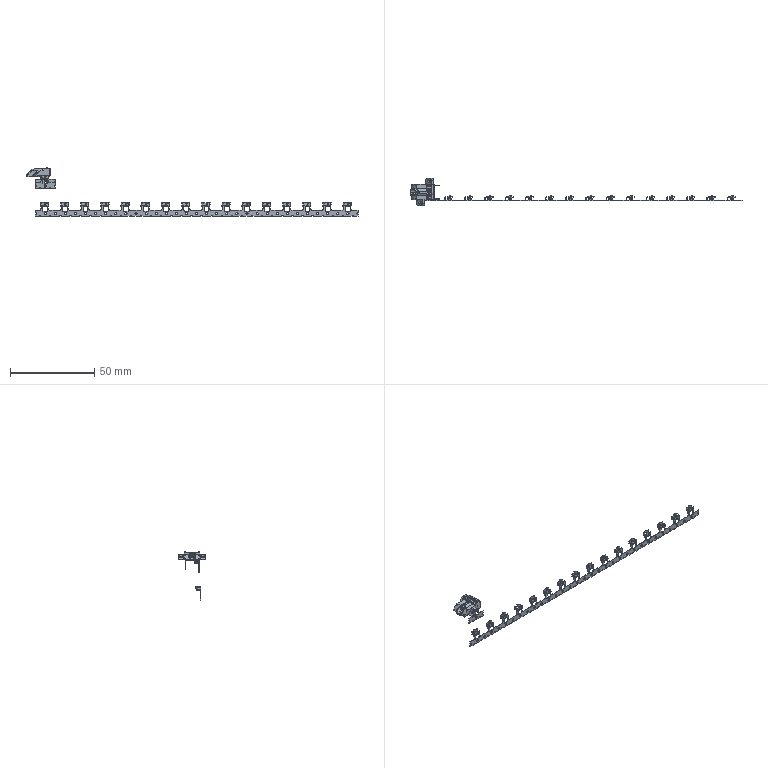Part | NX | 4 solids | 3674 faces | volume 566.334 mm3 | plane 2134 | cylinder 1174 | torus 246 | spline 54 | sphere 48 | cone 18 | commonest cylinder face diameters 0.3 x288 0.2 x206 0.7 x98 1.3 x93 0.5 x91 0.4 x84